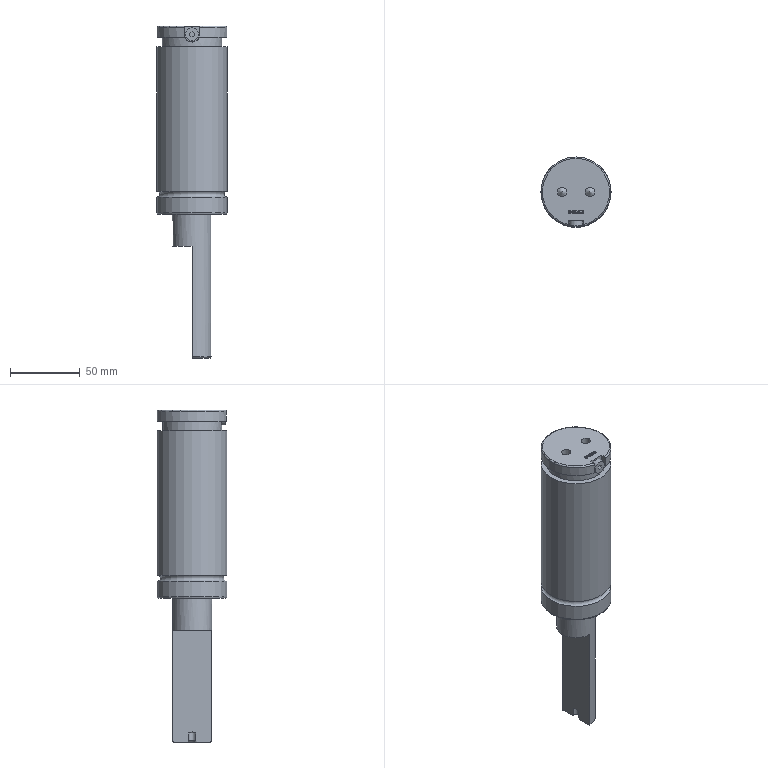Part | NX | features DG 2 | 1 solid | 169 faces | box 50.2 x 50.2 x 238 mm | volume 300026 mm3 | plane 127 | spline 24 | cylinder 10 | cone 4 | torus 4 | commonest cylinder face diameters 50.2 x3 6.6 x2 4.9 x1 9.5 x1 11 x1 28 x1